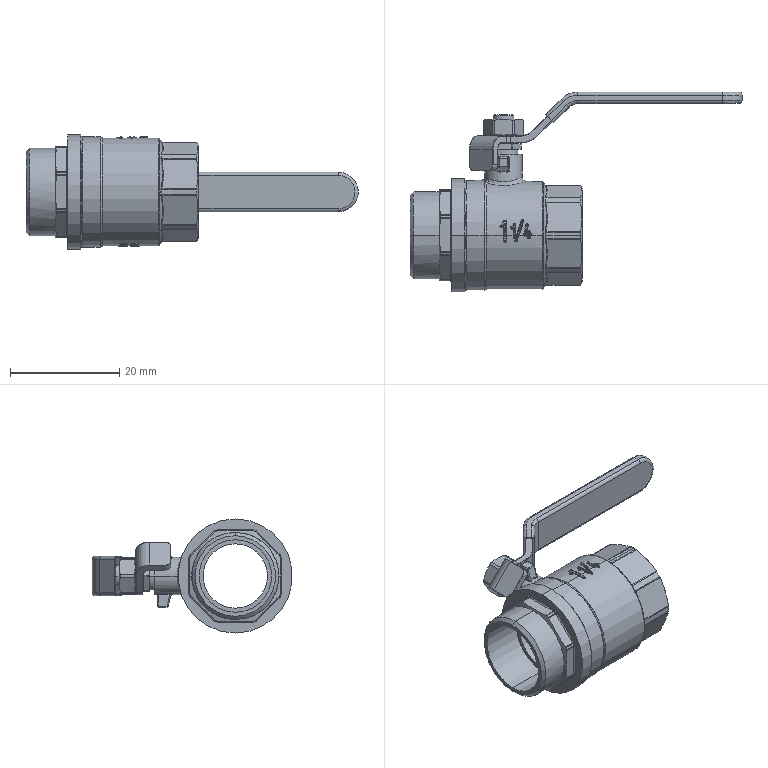Part | SolidWorks | features BaseBody 2, Scale 1 | 2 solids | 824 faces | box 60.8 x 36.67 x 20.9 mm | volume 5725 mm3 | spline 489 | cylinder 196 | plane 121 | cone 18 | commonest cylinder face diameters 0.152 x51 1.14 x40 0.38 x28 20.14 x14 18.24 x9 17.86 x8